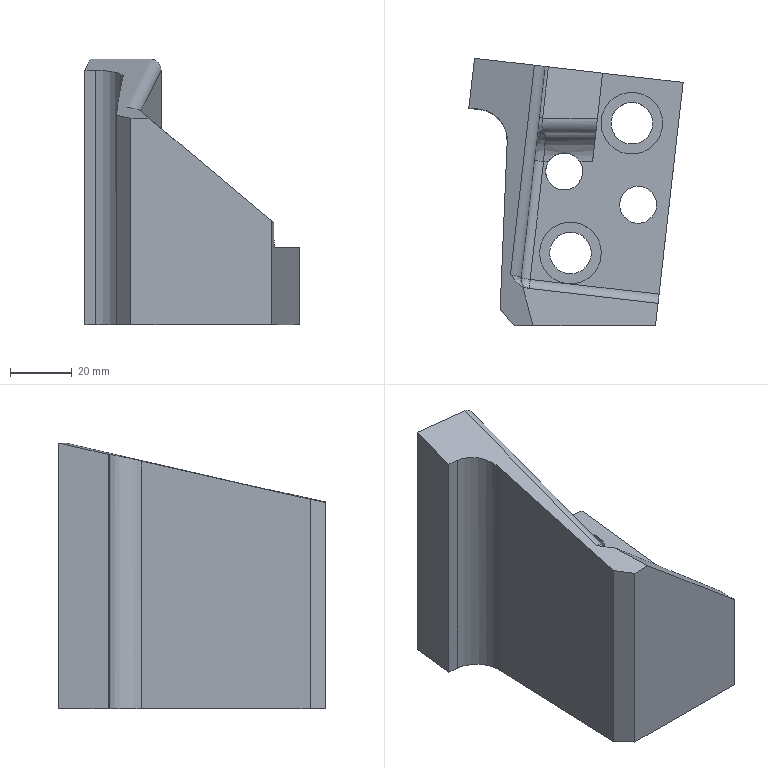Part | NX | features 23 2 | 1 solid | 37 faces | box 69.395 x 86.433 x 86.097 mm | volume 170408 mm3 | plane 18 | cylinder 15 | spline 3 | sphere 1 | commonest cylinder face diameters 6 x5 20 x3 12.001 x2 13.5 x2 7 x1 10 x1
STEP:
#1=CARTESIAN_POINT('',(3804.577,-393.184,-138.));
#2=VERTEX_POINT('',#1);
#3=CARTESIAN_POINT('',(3804.577,-393.184,-104.287));
#4=VERTEX_POINT('',#3);
#5=CARTESIAN_POINT('',(3804.577,-393.184,-83.583));
#6=DIRECTION('',(-0.000000001,0.,1.));
#7=VECTOR('',#6,1000.);
#8=LINE('',#5,#7);
#9=EDGE_CURVE('',#2,#4,#8,.T.);
#10=ORIENTED_EDGE('',*,*,#9,.F.);
#11=CARTESIAN_POINT('',(3813.548,-314.448,-138.));
#12=VERTEX_POINT('',#11);
#13=CARTESIAN_POINT('',(3842.238,-62.642,-138.));
#14=DIRECTION('',(0.1132,0.9936,0.));
#15=VECTOR('',#14,1000.);
#16=LINE('',#13,#15);
#17=EDGE_CURVE('',#2,#12,#16,.T.);
#18=ORIENTED_EDGE('',*,*,#17,.T.);
#19=CARTESIAN_POINT('',(3813.548,-314.448,-113.));
#20=VERTEX_POINT('',#19);
#21=CARTESIAN_POINT('',(3813.548,-314.448,-100.995));
#22=DIRECTION('',(0.000000001,0.,-1.));
#23=VECTOR('',#22,1000.);
#24=LINE('',#21,#23);
#25=EDGE_CURVE('',#20,#12,#24,.T.);
#26=ORIENTED_EDGE('',*,*,#25,.F.);
#27=CARTESIAN_POINT('',(3805.737,-383.004,-113.));
#28=VERTEX_POINT('',#27);
#29=CARTESIAN_POINT('',(3817.039,-283.812,-113.));
#30=DIRECTION('',(0.1132,0.9936,0.));
#31=VECTOR('',#30,1000.);
#32=LINE('',#29,#31);
#33=EDGE_CURVE('',#28,#20,#32,.T.);
#34=ORIENTED_EDGE('',*,*,#33,.F.);
#35=CARTESIAN_POINT('',(3805.397,-385.985,-110.));
#36=VERTEX_POINT('',#35);
#37=CARTESIAN_POINT('',(3805.737,-383.004,-110.));
#38=DIRECTION('',(-0.9936,0.1132,-0.000000001));
#39=DIRECTION('',(-0.1132,-0.9936,0.));
#40=AXIS2_PLACEMENT_3D('',#37,#38,#39);
#41=CIRCLE('',#40,3.);
#42=EDGE_CURVE('',#28,#36,#41,.T.);
#43=ORIENTED_EDGE('',*,*,#42,.T.);
#44=CARTESIAN_POINT('',(3805.397,-385.985,-104.975));
#45=VERTEX_POINT('',#44);
#46=CARTESIAN_POINT('',(3805.397,-385.985,-102.134));
#47=DIRECTION('',(0.000000001,0.,-1.));
#48=VECTOR('',#47,1000.);
#49=LINE('',#46,#48);
#50=EDGE_CURVE('',#45,#36,#49,.T.);
#51=ORIENTED_EDGE('',*,*,#50,.F.);
#52=CARTESIAN_POINT('',(3792.366,-500.365,-94.04));
#53=DIRECTION('',(-0.1127,-0.9891,0.09456));
#54=VECTOR('',#53,1000.);
#55=LINE('',#52,#54);
#56=EDGE_CURVE('',#45,#4,#55,.T.);
#57=ORIENTED_EDGE('',*,*,#56,.T.);
#58=EDGE_LOOP('',(#10,#18,#26,#34,#43,#51,#57));
#59=FACE_BOUND('',#58,.T.);
#60=CARTESIAN_POINT('',(3817.039,-283.812,-83.583));
#61=DIRECTION('',(-0.9936,0.1132,-0.000000001));
#62=DIRECTION('',(0.1132,0.9936,0.));
#63=AXIS2_PLACEMENT_3D('',#60,#61,#62);
#64=PLANE('',#63);
#65=ADVANCED_FACE('',(#59),#64,.F.);
#66=CARTESIAN_POINT('',(3754.275,-388.188,-138.));
#67=VERTEX_POINT('',#66);
#68=CARTESIAN_POINT('',(3756.561,-333.591,-138.));
#69=VERTEX_POINT('',#68);
#70=CARTESIAN_POINT('',(3774.796,101.868,-138.));
#71=DIRECTION('',(0.04184,0.9991,0.));
#72=VECTOR('',#71,1000.);
#73=LINE('',#70,#72);
#74=EDGE_CURVE('',#67,#69,#73,.T.);
#75=ORIENTED_EDGE('',*,*,#74,.F.);
#76=CARTESIAN_POINT('',(3754.275,-388.188,-70.123));
#77=VERTEX_POINT('',#76);
#78=CARTESIAN_POINT('',(3754.275,-388.188,-382.321));
#79=DIRECTION('',(0.,0.,1.));
#80=VECTOR('',#79,1000.);
#81=LINE('',#78,#80);
#82=EDGE_CURVE('',#67,#77,#81,.T.);
#83=ORIENTED_EDGE('',*,*,#82,.T.);
#84=CARTESIAN_POINT('',(3756.561,-333.591,-57.705));
#85=VERTEX_POINT('',#84);
#86=CARTESIAN_POINT('',(3754.968,-371.632,-66.358));
#87=DIRECTION('',(0.0408,0.9743,0.2216));
#88=VECTOR('',#87,1000.);
#89=LINE('',#86,#88);
#90=EDGE_CURVE('',#77,#85,#89,.T.);
#91=ORIENTED_EDGE('',*,*,#90,.T.);
#92=CARTESIAN_POINT('',(3756.561,-333.591,-133.));
#93=DIRECTION('',(0.,0.,-1.));
#94=VECTOR('',#93,1000.);
#95=LINE('',#92,#94);
#96=EDGE_CURVE('',#85,#69,#95,.T.);
#97=ORIENTED_EDGE('',*,*,#96,.T.);
#98=EDGE_LOOP('',(#75,#83,#91,#97));
#99=FACE_BOUND('',#98,.T.);
#100=CARTESIAN_POINT('',(3759.776,-256.811,-382.321));
#101=DIRECTION('',(-0.9991,0.04184,0.));
#102=DIRECTION('',(0.04184,0.9991,0.));
#103=AXIS2_PLACEMENT_3D('',#100,#101,#102);
#104=PLANE('',#103);
#105=ADVANCED_FACE('',(#99),#104,.T.);
#106=ORIENTED_EDGE('',*,*,#90,.F.);
#107=CARTESIAN_POINT('',(3759.066,-393.184,-71.13));
#108=VERTEX_POINT('',#107);
#109=CARTESIAN_POINT('',(3785.069,-420.298,-76.597));
#110=DIRECTION('',(0.6849,-0.7142,-0.144));
#111=VECTOR('',#110,1000.);
#112=LINE('',#109,#111);
#113=EDGE_CURVE('',#77,#108,#112,.T.);
#114=ORIENTED_EDGE('',*,*,#113,.T.);
#115=CARTESIAN_POINT('',(3764.884,-393.184,-70.98));
#116=VERTEX_POINT('',#115);
#117=CARTESIAN_POINT('',(3765.334,-393.184,-70.968));
#118=DIRECTION('',(-0.9997,0.,-0.02578));
#119=VECTOR('',#118,1000.);
#120=LINE('',#117,#119);
#121=EDGE_CURVE('',#116,#108,#120,.T.);
#122=ORIENTED_EDGE('',*,*,#121,.F.);
#123=CARTESIAN_POINT('',(3761.625,-380.732,-68.246));
#124=VERTEX_POINT('',#123);
#125=CARTESIAN_POINT('',(3784.867,-469.535,-87.747));
#126=DIRECTION('',(-0.2477,0.9463,0.2078));
#127=VECTOR('',#126,1000.);
#128=LINE('',#125,#127);
#129=EDGE_CURVE('',#116,#124,#128,.T.);
#130=ORIENTED_EDGE('',*,*,#129,.T.);
#131=CARTESIAN_POINT('',(3757.624,-376.852,-67.47));
#132=VERTEX_POINT('',#131);
#133=CARTESIAN_POINT('',(3761.625,-380.732,-68.246));
#134=CARTESIAN_POINT('',(3761.272,-380.557,-68.215));
#135=CARTESIAN_POINT('',(3760.738,-380.211,-68.151));
#136=CARTESIAN_POINT('',(3760.089,-379.642,-68.038));
#137=CARTESIAN_POINT('',(3759.731,-379.291,-67.968));
#138=CARTESIAN_POINT('',(3759.413,-378.954,-67.9));
#139=CARTESIAN_POINT('',(3759.272,-378.795,-67.868));
#140=CARTESIAN_POINT('',(3758.967,-378.446,-67.797));
#141=CARTESIAN_POINT('',(3758.665,-378.087,-67.723));
#142=CARTESIAN_POINT('',(3758.18,-377.503,-67.603));
#143=CARTESIAN_POINT('',(3757.844,-377.103,-67.522));
#144=CARTESIAN_POINT('',(3757.683,-376.916,-67.483));
#145=CARTESIAN_POINT('',(3757.624,-376.852,-67.47));
#146=B_SPLINE_CURVE_WITH_KNOTS('',3,(#133,#134,#135,#136,#137,#138,#139,#140,#141,#142,#143,#144,#145),.UNSPECIFIED.,.F.,.F.,(4,1,1,1,1,1,1,1,1,1,4),(0.,0.25,0.375,0.4375,0.5,0.5625,0.625,0.75,0.8125,0.875,1.),.UNSPECIFIED.);
#147=EDGE_CURVE('',#124,#132,#146,.T.);
#148=ORIENTED_EDGE('',*,*,#147,.T.);
#149=CARTESIAN_POINT('',(3765.36,-308.958,-51.903));
#150=VERTEX_POINT('',#149);
#151=CARTESIAN_POINT('',(3758.256,-371.305,-66.199));
#152=DIRECTION('',(-0.1104,-0.9687,-0.2221));
#153=VECTOR('',#152,1000.);
#154=LINE('',#151,#153);
#155=EDGE_CURVE('',#150,#132,#154,.T.);
#156=ORIENTED_EDGE('',*,*,#155,.F.);
#157=CARTESIAN_POINT('',(3745.985,-306.75,-51.903));
#158=VERTEX_POINT('',#157);
#159=CARTESIAN_POINT('',(3772.315,-309.75,-51.903));
#160=DIRECTION('',(0.9936,-0.1132,-0.000000001));
#161=VECTOR('',#160,1000.);
#162=LINE('',#159,#161);
#163=EDGE_CURVE('',#158,#150,#162,.T.);
#164=ORIENTED_EDGE('',*,*,#163,.F.);
#165=CARTESIAN_POINT('',(3744.153,-322.832,-55.59));
#166=VERTEX_POINT('',#165);
#167=CARTESIAN_POINT('',(3738.882,-369.098,-66.199));
#168=DIRECTION('',(-0.1104,-0.9687,-0.2221));
#169=VECTOR('',#168,1000.);
#170=LINE('',#167,#169);
#171=EDGE_CURVE('',#158,#166,#170,.T.);
#172=ORIENTED_EDGE('',*,*,#171,.T.);
#173=CARTESIAN_POINT('',(3747.702,-323.236,-55.59));
#174=VERTEX_POINT('',#173);
#175=CARTESIAN_POINT('',(3737.198,-322.04,-55.59));
#176=DIRECTION('',(0.9936,-0.1132,-0.000000001));
#177=VECTOR('',#176,1000.);
#178=LINE('',#175,#177);
#179=EDGE_CURVE('',#166,#174,#178,.T.);
#180=ORIENTED_EDGE('',*,*,#179,.T.);
#181=CARTESIAN_POINT('',(3746.57,-333.172,-57.868));
#182=DIRECTION('',(0.02515,0.2207,-0.975));
#183=DIRECTION('',(0.1104,0.9687,0.2221));
#184=AXIS2_PLACEMENT_3D('',#181,#182,#183);
#185=ELLIPSE('',#184,10.256,10.);
#186=EDGE_CURVE('',#174,#85,#185,.T.);
#187=ORIENTED_EDGE('',*,*,#186,.T.);
#188=EDGE_LOOP('',(#106,#114,#122,#130,#148,#156,#164,#172,#180,#187));
#189=FACE_BOUND('',#188,.T.);
#190=CARTESIAN_POINT('',(3765.211,-372.098,-66.199));
#191=DIRECTION('',(0.02515,0.2207,-0.975));
#192=DIRECTION('',(-0.1104,-0.9687,-0.2221));
#193=AXIS2_PLACEMENT_3D('',#190,#191,#192);
#194=PLANE('',#193);
#195=ADVANCED_FACE('',(#189),#194,.F.);
#196=CARTESIAN_POINT('',(3790.196,-327.653,-138.));
#197=VERTEX_POINT('',#196);
#198=CARTESIAN_POINT('',(3796.946,-327.653,-138.));
#199=DIRECTION('',(0.,0.,-1.));
#200=DIRECTION('',(-1.,0.,0.));
#201=AXIS2_PLACEMENT_3D('',#198,#199,#200);
#202=CIRCLE('',#201,6.75);
#203=EDGE_CURVE('',#197,#197,#202,.T.);
#204=ORIENTED_EDGE('',*,*,#203,.F.);
#205=EDGE_LOOP('',(#204));
#206=FACE_BOUND('',#205,.T.);
#207=CARTESIAN_POINT('',(3769.037,-343.274,-138.));
#208=VERTEX_POINT('',#207);
#209=CARTESIAN_POINT('',(3775.037,-343.274,-138.));
#210=DIRECTION('',(0.,0.,-1.));
#211=DIRECTION('',(-1.,0.,0.));
#212=AXIS2_PLACEMENT_3D('',#209,#210,#211);
#213=CIRCLE('',#212,6.);
#214=EDGE_CURVE('',#208,#208,#213,.T.);
#215=ORIENTED_EDGE('',*,*,#214,.F.);
#216=EDGE_LOOP('',(#215));
#217=FACE_BOUND('',#216,.T.);
#218=CARTESIAN_POINT('',(3792.971,-354.052,-138.));
#219=VERTEX_POINT('',#218);
#220=CARTESIAN_POINT('',(3798.971,-354.052,-138.));
#221=DIRECTION('',(0.,0.,-1.));
#222=DIRECTION('',(-1.,0.,0.));
#223=AXIS2_PLACEMENT_3D('',#220,#221,#222);
#224=CIRCLE('',#223,6.);
#225=EDGE_CURVE('',#219,#219,#224,.T.);
#226=ORIENTED_EDGE('',*,*,#225,.F.);
#227=EDGE_LOOP('',(#226));
#228=FACE_BOUND('',#227,.T.);
#229=CARTESIAN_POINT('',(3770.312,-369.673,-138.));
#230=VERTEX_POINT('',#229);
#231=CARTESIAN_POINT('',(3777.062,-369.673,-138.));
#232=DIRECTION('',(0.,0.,-1.));
#233=DIRECTION('',(-1.,0.,0.));
#234=AXIS2_PLACEMENT_3D('',#231,#232,#233);
#235=CIRCLE('',#234,6.75);
#236=EDGE_CURVE('',#230,#230,#235,.T.);
#237=ORIENTED_EDGE('',*,*,#236,.F.);
#238=EDGE_LOOP('',(#237));
#239=FACE_BOUND('',#238,.T.);
#240=CARTESIAN_POINT('',(3759.066,-393.184,-138.));
#241=VERTEX_POINT('',#240);
#242=CARTESIAN_POINT('',(1598.5,-393.184,-138.));
#243=DIRECTION('',(-1.,0.,0.));
#244=VECTOR('',#243,1000.);
#245=LINE('',#242,#244);
#246=EDGE_CURVE('',#2,#241,#245,.T.);
#247=ORIENTED_EDGE('',*,*,#246,.T.);
#248=CARTESIAN_POINT('',(2431.145,991.508,-138.));
#249=DIRECTION('',(-0.6922,0.7217,0.));
#250=VECTOR('',#249,1000.);
#251=LINE('',#248,#250);
#252=EDGE_CURVE('',#241,#67,#251,.T.);
#253=ORIENTED_EDGE('',*,*,#252,.T.);
#254=ORIENTED_EDGE('',*,*,#74,.T.);
#255=CARTESIAN_POINT('',(3747.702,-323.236,-138.));
#256=VERTEX_POINT('',#255);
#257=CARTESIAN_POINT('',(3746.57,-333.172,-138.));
#258=DIRECTION('',(0.,0.,1.));
#259=DIRECTION('',(-1.,0.,0.));
#260=AXIS2_PLACEMENT_3D('',#257,#258,#259);
#261=CIRCLE('',#260,10.);
#262=EDGE_CURVE('',#69,#256,#261,.T.);
#263=ORIENTED_EDGE('',*,*,#262,.T.);
#264=CARTESIAN_POINT('',(3744.153,-322.832,-138.));
#265=VERTEX_POINT('',#264);
#266=CARTESIAN_POINT('',(3737.198,-322.04,-138.));
#267=DIRECTION('',(0.9936,-0.1132,0.));
#268=VECTOR('',#267,1000.);
#269=LINE('',#266,#268);
#270=EDGE_CURVE('',#265,#256,#269,.T.);
#271=ORIENTED_EDGE('',*,*,#270,.F.);
#272=CARTESIAN_POINT('',(3745.985,-306.75,-138.));
#273=VERTEX_POINT('',#272);
#274=CARTESIAN_POINT('',(3774.675,-54.944,-138.));
#275=DIRECTION('',(-0.1132,-0.9936,0.));
#276=VECTOR('',#275,1000.);
#277=LINE('',#274,#276);
#278=EDGE_CURVE('',#273,#265,#277,.T.);
#279=ORIENTED_EDGE('',*,*,#278,.F.);
#280=CARTESIAN_POINT('',(1569.81,-58.806,-138.));
#281=DIRECTION('',(0.9936,-0.1132,0.));
#282=VECTOR('',#281,1000.);
#283=LINE('',#280,#282);
#284=EDGE_CURVE('',#273,#12,#283,.T.);
#285=ORIENTED_EDGE('',*,*,#284,.T.);
#286=ORIENTED_EDGE('',*,*,#17,.F.);
#287=EDGE_LOOP('',(#247,#253,#254,#263,#271,#279,#285,#286));
#288=FACE_BOUND('',#287,.T.);
#289=CARTESIAN_POINT('',(1598.5,193.,-138.));
#290=DIRECTION('',(0.,0.,-1.));
#291=DIRECTION('',(-1.,0.,0.));
#292=AXIS2_PLACEMENT_3D('',#289,#290,#291);
#293=PLANE('',#292);
#294=ADVANCED_FACE('',(#206,#217,#228,#239,#288),#293,.T.);
#295=ORIENTED_EDGE('',*,*,#129,.F.);
#296=CARTESIAN_POINT('',(3738.981,-393.184,-49.245));
#297=DIRECTION('',(0.766,0.,-0.6428));
#298=VECTOR('',#297,1000.);
#299=LINE('',#296,#298);
#300=EDGE_CURVE('',#116,#4,#299,.T.);
#301=ORIENTED_EDGE('',*,*,#300,.T.);
#302=ORIENTED_EDGE('',*,*,#56,.F.);
#303=CARTESIAN_POINT('',(3763.53,-381.215,-69.844));
#304=VERTEX_POINT('',#303);
#305=CARTESIAN_POINT('',(3746.385,-379.261,-55.457));
#306=DIRECTION('',(0.7631,-0.08695,-0.6404));
#307=VECTOR('',#306,1000.);
#308=LINE('',#305,#307);
#309=EDGE_CURVE('',#304,#45,#308,.T.);
#310=ORIENTED_EDGE('',*,*,#309,.F.);
#311=CARTESIAN_POINT('',(3763.53,-381.215,-69.844));
#312=CARTESIAN_POINT('',(3762.882,-381.141,-69.3));
#313=CARTESIAN_POINT('',(3762.255,-380.926,-68.774));
#314=CARTESIAN_POINT('',(3761.625,-380.733,-68.245));
#315=B_SPLINE_CURVE_WITH_KNOTS('',3,(#311,#312,#313,#314),.UNSPECIFIED.,.F.,.F.,(4,4),(0.,0.002533),.UNSPECIFIED.);
#316=EDGE_CURVE('',#304,#124,#315,.T.);
#317=ORIENTED_EDGE('',*,*,#316,.T.);
#318=EDGE_LOOP('',(#295,#301,#302,#310,#317));
#319=FACE_BOUND('',#318,.T.);
#320=CARTESIAN_POINT('',(3738.981,-490.,-49.245));
#321=DIRECTION('',(0.6428,0.,0.766));
#322=DIRECTION('',(-0.766,0.,0.6428));
#323=AXIS2_PLACEMENT_3D('',#320,#321,#322);
#324=PLANE('',#323);
#325=ADVANCED_FACE('',(#319),#324,.T.);
#326=CARTESIAN_POINT('',(3786.946,-327.653,-128.));
#327=VERTEX_POINT('',#326);
#328=CARTESIAN_POINT('',(3796.946,-327.653,-128.));
#329=DIRECTION('',(0.,0.,-1.));
#330=DIRECTION('',(-1.,0.,0.));
#331=AXIS2_PLACEMENT_3D('',#328,#329,#330);
#332=CIRCLE('',#331,10.);
#333=EDGE_CURVE('',#327,#327,#332,.T.);
#334=ORIENTED_EDGE('',*,*,#333,.T.);
#335=EDGE_LOOP('',(#334));
#336=FACE_BOUND('',#335,.T.);
#337=CARTESIAN_POINT('',(3786.946,-327.653,-113.));
#338=VERTEX_POINT('',#337);
#339=CARTESIAN_POINT('',(3796.946,-327.653,-113.));
#340=DIRECTION('',(0.,0.,1.));
#341=DIRECTION('',(-1.,0.,0.));
#342=AXIS2_PLACEMENT_3D('',#339,#340,#341);
#343=CIRCLE('',#342,10.);
#344=EDGE_CURVE('',#338,#338,#343,.T.);
#345=ORIENTED_EDGE('',*,*,#344,.T.);
#346=EDGE_LOOP('',(#345));
#347=FACE_BOUND('',#346,.T.);
#348=CARTESIAN_POINT('',(3796.946,-327.653,-103.074));
#349=DIRECTION('',(0.,0.,-1.));
#350=DIRECTION('',(-1.,0.,0.));
#351=AXIS2_PLACEMENT_3D('',#348,#349,#350);
#352=CYLINDRICAL_SURFACE('',#351,10.);
#353=ADVANCED_FACE('',(#336,#347),#352,.F.);
#354=ORIENTED_EDGE('',*,*,#344,.F.);
#355=EDGE_LOOP('',(#354));
#356=FACE_BOUND('',#355,.T.);
#357=CARTESIAN_POINT('',(3792.971,-354.052,-113.));
#358=VERTEX_POINT('',#357);
#359=CARTESIAN_POINT('',(3798.971,-354.052,-113.));
#360=DIRECTION('',(0.,0.,1.));
#361=DIRECTION('',(-1.,0.,0.));
#362=AXIS2_PLACEMENT_3D('',#359,#360,#361);
#363=CIRCLE('',#362,6.);
#364=EDGE_CURVE('',#358,#358,#363,.T.);
#365=ORIENTED_EDGE('',*,*,#364,.F.);
#366=EDGE_LOOP('',(#365));
#367=FACE_BOUND('',#366,.T.);
#368=CARTESIAN_POINT('',(3768.354,-340.096,-113.));
#369=VERTEX_POINT('',#368);
#370=CARTESIAN_POINT('',(3769.947,-340.096,-113.));
#371=VERTEX_POINT('',#370);
#372=CARTESIAN_POINT('',(282.5,-340.096,-113.));
#373=DIRECTION('',(1.,0.,0.));
#374=VECTOR('',#373,1000.);
#375=LINE('',#372,#374);
#376=EDGE_CURVE('',#369,#371,#375,.T.);
#377=ORIENTED_EDGE('',*,*,#376,.F.);
#378=CARTESIAN_POINT('',(3764.007,-378.25,-113.));
#379=VERTEX_POINT('',#378);
#380=CARTESIAN_POINT('',(3764.007,-378.25,-113.));
#381=DIRECTION('',(-0.1132,-0.9936,0.));
#382=VECTOR('',#381,1000.);
#383=LINE('',#380,#382);
#384=EDGE_CURVE('',#369,#379,#383,.T.);
#385=ORIENTED_EDGE('',*,*,#384,.T.);
#386=CARTESIAN_POINT('',(3775.93,-379.608,-113.));
#387=VERTEX_POINT('',#386);
#388=CARTESIAN_POINT('',(262.864,20.655,-113.));
#389=DIRECTION('',(0.9936,-0.1132,0.));
#390=VECTOR('',#389,1000.);
#391=LINE('',#388,#390);
#392=EDGE_CURVE('',#379,#387,#391,.T.);
#393=ORIENTED_EDGE('',*,*,#392,.T.);
#394=CARTESIAN_POINT('',(3777.062,-369.673,-113.));
#395=DIRECTION('',(0.,0.,1.));
#396=DIRECTION('',(-1.,0.,0.));
#397=AXIS2_PLACEMENT_3D('',#394,#395,#396);
#398=CIRCLE('',#397,10.);
#399=EDGE_CURVE('',#387,#387,#398,.T.);
#400=ORIENTED_EDGE('',*,*,#399,.F.);
#401=CARTESIAN_POINT('',(262.864,20.655,-113.));
#402=DIRECTION('',(0.9936,-0.1132,0.));
#403=VECTOR('',#402,1000.);
#404=LINE('',#401,#403);
#405=EDGE_CURVE('',#387,#28,#404,.T.);
#406=ORIENTED_EDGE('',*,*,#405,.T.);
#407=ORIENTED_EDGE('',*,*,#33,.T.);
#408=CARTESIAN_POINT('',(3787.453,-311.475,-113.));
#409=VERTEX_POINT('',#408);
#410=CARTESIAN_POINT('',(3780.809,-310.718,-113.));
#411=DIRECTION('',(-0.9936,0.1132,0.));
#412=VECTOR('',#411,1000.);
#413=LINE('',#410,#412);
#414=EDGE_CURVE('',#20,#409,#413,.T.);
#415=ORIENTED_EDGE('',*,*,#414,.T.);
#416=CARTESIAN_POINT('',(3784.192,-340.096,-113.));
#417=VERTEX_POINT('',#416);
#418=CARTESIAN_POINT('',(3799.278,-207.685,-113.));
#419=DIRECTION('',(-0.1132,-0.9936,0.));
#420=VECTOR('',#419,1000.);
#421=LINE('',#418,#420);
#422=EDGE_CURVE('',#409,#417,#421,.T.);
#423=ORIENTED_EDGE('',*,*,#422,.T.);
#424=CARTESIAN_POINT('',(3780.128,-340.096,-113.));
#425=VERTEX_POINT('',#424);
#426=CARTESIAN_POINT('',(282.5,-340.096,-113.));
#427=DIRECTION('',(1.,0.,0.));
#428=VECTOR('',#427,1000.);
#429=LINE('',#426,#428);
#430=EDGE_CURVE('',#425,#417,#429,.T.);
#431=ORIENTED_EDGE('',*,*,#430,.F.);
#432=CARTESIAN_POINT('',(3775.037,-343.274,-113.));
#433=DIRECTION('',(0.,0.,1.));
#434=DIRECTION('',(-1.,0.,0.));
#435=AXIS2_PLACEMENT_3D('',#432,#433,#434);
#436=CIRCLE('',#435,6.);
#437=EDGE_CURVE('',#371,#425,#436,.T.);
#438=ORIENTED_EDGE('',*,*,#437,.F.);
#439=EDGE_LOOP('',(#377,#385,#393,#400,#406,#407,#415,#423,#431,#438));
#440=FACE_BOUND('',#439,.T.);
#441=CARTESIAN_POINT('',(282.5,193.,-113.));
#442=DIRECTION('',(0.,0.,-1.));
#443=DIRECTION('',(-1.,0.,0.));
#444=AXIS2_PLACEMENT_3D('',#441,#442,#443);
#445=PLANE('',#444);
#446=ADVANCED_FACE('',(#356,#367,#440),#445,.F.);
#447=CARTESIAN_POINT('',(3787.453,-311.475,-91.917));
#448=VERTEX_POINT('',#447);
#449=CARTESIAN_POINT('',(3769.914,-309.477,-77.201));
#450=VERTEX_POINT('',#449);
#451=CARTESIAN_POINT('',(3788.947,-311.645,-93.171));
#452=DIRECTION('',(-0.7631,0.08695,0.6404));
#453=VECTOR('',#452,1000.);
#454=LINE('',#451,#453);
#455=EDGE_CURVE('',#448,#450,#454,.T.);
#456=ORIENTED_EDGE('',*,*,#455,.T.);
#457=CARTESIAN_POINT('',(3768.021,-326.096,-75.612));
#458=VERTEX_POINT('',#457);
#459=CARTESIAN_POINT('',(3635.355,-1490.486,35.707));
#460=DIRECTION('',(-0.1127,-0.9891,0.09456));
#461=VECTOR('',#460,1000.);
#462=LINE('',#459,#461);
#463=EDGE_CURVE('',#450,#458,#462,.T.);
#464=ORIENTED_EDGE('',*,*,#463,.T.);
#465=CARTESIAN_POINT('',(3785.787,-326.096,-90.52));
#466=VERTEX_POINT('',#465);
#467=CARTESIAN_POINT('',(3738.981,-326.096,-51.245));
#468=DIRECTION('',(0.766,0.,-0.6428));
#469=VECTOR('',#468,1000.);
#470=LINE('',#467,#469);
#471=EDGE_CURVE('',#458,#466,#470,.T.);
#472=ORIENTED_EDGE('',*,*,#471,.T.);
#473=CARTESIAN_POINT('',(3766.504,-495.344,-74.339));
#474=DIRECTION('',(-0.1127,-0.9891,0.09456));
#475=VECTOR('',#474,1000.);
#476=LINE('',#473,#475);
#477=EDGE_CURVE('',#448,#466,#476,.T.);
#478=ORIENTED_EDGE('',*,*,#477,.F.);
#479=EDGE_LOOP('',(#456,#464,#472,#478));
#480=FACE_BOUND('',#479,.T.);
#481=CARTESIAN_POINT('',(3738.981,-490.,-51.245));
#482=DIRECTION('',(0.6428,0.,0.766));
#483=DIRECTION('',(-0.766,0.,0.6428));
#484=AXIS2_PLACEMENT_3D('',#481,#482,#483);
#485=PLANE('',#484);
#486=ADVANCED_FACE('',(#480),#485,.T.);
#487=CARTESIAN_POINT('',(3787.453,-311.475,-100.995));
#488=DIRECTION('',(0.,0.,-1.));
#489=VECTOR('',#488,1000.);
#490=LINE('',#487,#489);
#491=EDGE_CURVE('',#448,#409,#490,.T.);
#492=ORIENTED_EDGE('',*,*,#491,.T.);
#493=ORIENTED_EDGE('',*,*,#414,.F.);
#494=ORIENTED_EDGE('',*,*,#25,.T.);
#495=ORIENTED_EDGE('',*,*,#284,.F.);
#496=CARTESIAN_POINT('',(3745.985,-306.75,-706.6));
#497=DIRECTION('',(0.000000001,0.,-1.));
#498=VECTOR('',#497,1000.);
#499=LINE('',#496,#498);
#500=EDGE_CURVE('',#158,#273,#499,.T.);
#501=ORIENTED_EDGE('',*,*,#500,.F.);
#502=ORIENTED_EDGE('',*,*,#163,.T.);
#503=CARTESIAN_POINT('',(3768.837,-309.354,-55.492));
#504=VERTEX_POINT('',#503);
#505=CARTESIAN_POINT('',(3765.36,-308.958,-55.492));
#506=DIRECTION('',(-0.1132,-0.9936,0.));
#507=DIRECTION('',(0.,0.,1.));
#508=AXIS2_PLACEMENT_3D('',#505,#506,#507);
#509=ELLIPSE('',#508,3.59,3.5);
#510=EDGE_CURVE('',#504,#150,#509,.T.);
#511=ORIENTED_EDGE('',*,*,#510,.F.);
#512=CARTESIAN_POINT('',(3768.837,-309.354,-74.882));
#513=VERTEX_POINT('',#512);
#514=CARTESIAN_POINT('',(3768.837,-309.354,-706.6));
#515=DIRECTION('',(-0.000000001,0.,1.));
#516=VECTOR('',#515,1000.);
#517=LINE('',#514,#516);
#518=EDGE_CURVE('',#513,#504,#517,.T.);
#519=ORIENTED_EDGE('',*,*,#518,.F.);
#520=CARTESIAN_POINT('',(3771.818,-309.693,-74.882));
#521=DIRECTION('',(-0.1132,-0.9936,0.));
#522=DIRECTION('',(-0.000000001,0.,1.));
#523=AXIS2_PLACEMENT_3D('',#520,#521,#522);
#524=ELLIPSE('',#523,3.014,3.);
#525=EDGE_CURVE('',#513,#450,#524,.T.);
#526=ORIENTED_EDGE('',*,*,#525,.T.);
#527=ORIENTED_EDGE('',*,*,#455,.F.);
#528=EDGE_LOOP('',(#492,#493,#494,#495,#501,#502,#511,#519,#526,#527));
#529=FACE_BOUND('',#528,.T.);
#530=CARTESIAN_POINT('',(3780.809,-310.718,-100.995));
#531=DIRECTION('',(-0.1132,-0.9936,0.));
#532=DIRECTION('',(-0.9936,0.1132,0.));
#533=AXIS2_PLACEMENT_3D('',#530,#531,#532);
#534=PLANE('',#533);
#535=ADVANCED_FACE('',(#529),#534,.F.);
#536=CARTESIAN_POINT('',(3785.217,-331.096,-96.569));
#537=VERTEX_POINT('',#536);
#538=CARTESIAN_POINT('',(3769.038,-331.096,-82.992));
#539=VERTEX_POINT('',#538);
#540=CARTESIAN_POINT('',(3769.312,-331.096,-83.222));
#541=DIRECTION('',(-0.766,0.,0.6428));
#542=VECTOR('',#541,1000.);
#543=LINE('',#540,#542);
#544=EDGE_CURVE('',#537,#539,#543,.T.);
#545=ORIENTED_EDGE('',*,*,#544,.T.);
#546=CARTESIAN_POINT('',(3769.038,-331.096,-104.));
#547=VERTEX_POINT('',#546);
#548=CARTESIAN_POINT('',(3769.038,-331.096,-104.));
#549=DIRECTION('',(0.000000001,0.,-1.));
#550=VECTOR('',#549,1000.);
#551=LINE('',#548,#550);
#552=EDGE_CURVE('',#539,#547,#551,.T.);
#553=ORIENTED_EDGE('',*,*,#552,.T.);
#554=CARTESIAN_POINT('',(3785.217,-331.096,-104.));
#555=VERTEX_POINT('',#554);
#556=CARTESIAN_POINT('',(3769.38,-331.096,-104.));
#557=DIRECTION('',(1.,0.,0.));
#558=VECTOR('',#557,1000.);
#559=LINE('',#556,#558);
#560=EDGE_CURVE('',#547,#555,#559,.T.);
#561=ORIENTED_EDGE('',*,*,#560,.T.);
#562=CARTESIAN_POINT('',(3785.217,-331.096,-81.141));
#563=DIRECTION('',(0.,0.,-1.));
#564=VECTOR('',#563,1000.);
#565=LINE('',#562,#564);
#566=EDGE_CURVE('',#537,#555,#565,.T.);
#567=ORIENTED_EDGE('',*,*,#566,.F.);
#568=EDGE_LOOP('',(#545,#553,#561,#567));
#569=FACE_BOUND('',#568,.T.);
#570=CARTESIAN_POINT('',(3769.38,-331.096,-81.141));
#571=DIRECTION('',(0.,-1.,0.));
#572=DIRECTION('',(0.,0.,1.));
#573=AXIS2_PLACEMENT_3D('',#570,#571,#572);
#574=PLANE('',#573);
#575=ADVANCED_FACE('',(#569),#574,.T.);
#576=CARTESIAN_POINT('',(3761.026,-377.91,-71.212));
#577=VERTEX_POINT('',#576);
#578=CARTESIAN_POINT('',(3617.366,-1638.801,-360.329));
#579=DIRECTION('',(0.1104,0.9687,0.2221));
#580=VECTOR('',#579,1000.);
#581=LINE('',#578,#580);
#582=EDGE_CURVE('',#577,#504,#581,.T.);
#583=ORIENTED_EDGE('',*,*,#582,.F.);
#584=CARTESIAN_POINT('',(3761.026,-377.91,-110.));
#585=VERTEX_POINT('',#584);
#586=CARTESIAN_POINT('',(3761.026,-377.91,-706.6));
#587=DIRECTION('',(0.000000001,0.,-1.));
#588=VECTOR('',#587,1000.);
#589=LINE('',#586,#588);
#590=EDGE_CURVE('',#577,#585,#589,.T.);
#591=ORIENTED_EDGE('',*,*,#590,.T.);
#592=CARTESIAN_POINT('',(3765.373,-339.757,-110.));
#593=VERTEX_POINT('',#592);
#594=CARTESIAN_POINT('',(3626.296,-1560.421,-110.));
#595=DIRECTION('',(0.1132,0.9936,0.));
#596=VECTOR('',#595,1000.);
#597=LINE('',#594,#596);
#598=EDGE_CURVE('',#585,#593,#597,.T.);
#599=ORIENTED_EDGE('',*,*,#598,.T.);
#600=CARTESIAN_POINT('',(3766.057,-333.757,-104.));
#601=VERTEX_POINT('',#600);
#602=CARTESIAN_POINT('',(3765.373,-339.757,-104.));
#603=DIRECTION('',(0.9936,-0.1132,0.000000001));
#604=DIRECTION('',(0.1132,0.9936,-0.000000007));
#605=AXIS2_PLACEMENT_3D('',#602,#603,#604);
#606=ELLIPSE('',#605,6.039,6.);
#607=EDGE_CURVE('',#593,#601,#606,.T.);
#608=ORIENTED_EDGE('',*,*,#607,.T.);
#609=CARTESIAN_POINT('',(3766.057,-333.757,-82.992));
#610=VERTEX_POINT('',#609);
#611=CARTESIAN_POINT('',(3766.057,-333.757,-78.746));
#612=DIRECTION('',(-0.000000001,0.,1.));
#613=VECTOR('',#612,1000.);
#614=LINE('',#611,#613);
#615=EDGE_CURVE('',#601,#610,#614,.T.);
#616=ORIENTED_EDGE('',*,*,#615,.T.);
#617=CARTESIAN_POINT('',(3766.968,-325.757,-73.314));
#618=VERTEX_POINT('',#617);
#619=CARTESIAN_POINT('',(3766.968,-325.757,-83.757));
#620=DIRECTION('',(-0.9936,0.1132,-0.000000001));
#621=DIRECTION('',(-0.01514,-0.1328,0.991));
#622=AXIS2_PLACEMENT_3D('',#619,#620,#621);
#623=ELLIPSE('',#622,10.511,8.);
#624=EDGE_CURVE('',#610,#618,#623,.T.);
#625=ORIENTED_EDGE('',*,*,#624,.T.);
#626=CARTESIAN_POINT('',(3634.303,-1490.146,38.006));
#627=DIRECTION('',(0.1127,0.9891,-0.09456));
#628=VECTOR('',#627,1000.);
#629=LINE('',#626,#628);
#630=EDGE_CURVE('',#618,#513,#629,.T.);
#631=ORIENTED_EDGE('',*,*,#630,.T.);
#632=ORIENTED_EDGE('',*,*,#518,.T.);
#633=EDGE_LOOP('',(#583,#591,#599,#608,#616,#625,#631,#632));
#634=FACE_BOUND('',#633,.T.);
#635=CARTESIAN_POINT('',(3626.296,-1560.421,-706.6));
#636=DIRECTION('',(0.9936,-0.1132,0.000000001));
#637=DIRECTION('',(0.000000001,0.000000001,-1.));
#638=AXIS2_PLACEMENT_3D('',#635,#636,#637);
#639=PLANE('',#638);
#640=ADVANCED_FACE('',(#634),#639,.T.);
#641=ORIENTED_EDGE('',*,*,#155,.T.);
#642=CARTESIAN_POINT('',(3757.624,-376.852,-67.47));
#643=CARTESIAN_POINT('',(3758.055,-376.901,-67.47));
#644=CARTESIAN_POINT('',(3758.723,-377.005,-67.611));
#645=CARTESIAN_POINT('',(3759.521,-377.172,-68.047));
#646=CARTESIAN_POINT('',(3760.117,-377.338,-68.6));
#647=CARTESIAN_POINT('',(3760.377,-377.433,-68.95));
#648=CARTESIAN_POINT('',(3760.834,-377.633,-69.739));
#649=CARTESIAN_POINT('',(3761.039,-377.796,-70.566));
#650=CARTESIAN_POINT('',(3761.026,-377.91,-71.212));
#651=B_SPLINE_CURVE_WITH_KNOTS('',3,(#642,#643,#644,#645,#646,#647,#648,#649,#650),.UNSPECIFIED.,.F.,.F.,(4,1,1,1,1,1,4),(0.,0.25,0.375,0.5,0.625,0.75,1.),.UNSPECIFIED.);
#652=EDGE_CURVE('',#132,#577,#651,.T.);
#653=ORIENTED_EDGE('',*,*,#652,.T.);
#654=ORIENTED_EDGE('',*,*,#582,.T.);
#655=ORIENTED_EDGE('',*,*,#510,.T.);
#656=EDGE_LOOP('',(#641,#653,#654,#655));
#657=FACE_BOUND('',#656,.T.);
#658=CARTESIAN_POINT('',(3768.744,-279.254,-48.681));
#659=DIRECTION('',(0.1104,0.9687,0.2221));
#660=DIRECTION('',(0.6848,-0.2361,0.6894));
#661=AXIS2_PLACEMENT_3D('',#658,#659,#660);
#662=CYLINDRICAL_SURFACE('',#661,3.5);
#663=ADVANCED_FACE('',(#657),#662,.T.);
#664=ORIENTED_EDGE('',*,*,#270,.T.);
#665=CARTESIAN_POINT('',(3747.702,-323.236,-382.321));
#666=DIRECTION('',(0.,0.,1.));
#667=VECTOR('',#666,1000.);
#668=LINE('',#665,#667);
#669=EDGE_CURVE('',#256,#174,#668,.T.);
#670=ORIENTED_EDGE('',*,*,#669,.T.);
#671=ORIENTED_EDGE('',*,*,#179,.F.);
#672=CARTESIAN_POINT('',(3744.153,-322.832,-706.6));
#673=DIRECTION('',(0.000000001,0.,-1.));
#674=VECTOR('',#673,1000.);
#675=LINE('',#672,#674);
#676=EDGE_CURVE('',#166,#265,#675,.T.);
#677=ORIENTED_EDGE('',*,*,#676,.T.);
#678=EDGE_LOOP('',(#664,#670,#671,#677));
#679=FACE_BOUND('',#678,.T.);
#680=CARTESIAN_POINT('',(3737.198,-322.04,-133.));
#681=DIRECTION('',(-0.1132,-0.9936,0.));
#682=DIRECTION('',(-0.9936,0.1132,0.));
#683=AXIS2_PLACEMENT_3D('',#680,#681,#682);
#684=PLANE('',#683);
#685=ADVANCED_FACE('',(#679),#684,.T.);
#686=ORIENTED_EDGE('',*,*,#186,.F.);
#687=ORIENTED_EDGE('',*,*,#669,.F.);
#688=ORIENTED_EDGE('',*,*,#262,.F.);
#689=ORIENTED_EDGE('',*,*,#96,.F.);
#690=EDGE_LOOP('',(#686,#687,#688,#689));
#691=FACE_BOUND('',#690,.T.);
#692=CARTESIAN_POINT('',(3746.57,-333.172,-382.321));
#693=DIRECTION('',(0.,0.,1.));
#694=DIRECTION('',(-1.,0.,0.));
#695=AXIS2_PLACEMENT_3D('',#692,#693,#694);
#696=CYLINDRICAL_SURFACE('',#695,10.);
#697=ADVANCED_FACE('',(#691),#696,.F.);
#698=ORIENTED_EDGE('',*,*,#171,.F.);
#699=ORIENTED_EDGE('',*,*,#500,.T.);
#700=ORIENTED_EDGE('',*,*,#278,.T.);
#701=ORIENTED_EDGE('',*,*,#676,.F.);
#702=EDGE_LOOP('',(#698,#699,#700,#701));
#703=FACE_BOUND('',#702,.T.);
#704=CARTESIAN_POINT('',(3603.444,-1557.817,-706.6));
#705=DIRECTION('',(0.9936,-0.1132,0.000000001));
#706=DIRECTION('',(0.000000001,0.000000001,-1.));
#707=AXIS2_PLACEMENT_3D('',#704,#705,#706);
#708=PLANE('',#707);
#709=ADVANCED_FACE('',(#703),#708,.F.);
#710=ORIENTED_EDGE('',*,*,#560,.F.);
#711=CARTESIAN_POINT('',(3769.038,-331.096,-104.));
#712=CARTESIAN_POINT('',(3769.038,-331.096,-105.113));
#713=CARTESIAN_POINT('',(3769.012,-331.413,-106.838));
#714=CARTESIAN_POINT('',(3768.94,-332.375,-108.696));
#715=CARTESIAN_POINT('',(3768.892,-333.014,-109.567));
#716=CARTESIAN_POINT('',(3768.863,-333.4,-110.021));
#717=CARTESIAN_POINT('',(3768.835,-333.763,-110.398));
#718=CARTESIAN_POINT('',(3768.821,-333.943,-110.569));
#719=CARTESIAN_POINT('',(3768.795,-334.28,-110.876));
#720=CARTESIAN_POINT('',(3768.746,-334.914,-111.385));
#721=CARTESIAN_POINT('',(3768.657,-336.07,-112.115));
#722=CARTESIAN_POINT('',(3768.522,-337.861,-112.798));
#723=CARTESIAN_POINT('',(3768.413,-339.319,-113.));
#724=CARTESIAN_POINT('',(3768.354,-340.096,-113.));
#725=B_SPLINE_CURVE_WITH_KNOTS('',3,(#711,#712,#713,#714,#715,#716,#717,#718,#719,#720,#721,#722,#723,#724),.UNSPECIFIED.,.F.,.F.,(4,1,1,1,1,1,1,1,1,1,1,4),(0.,0.25,0.375,0.4375,0.4688,0.5,0.5312,0.5625,0.625,0.75,0.875,1.),.UNSPECIFIED.);
#726=EDGE_CURVE('',#547,#369,#725,.T.);
#727=ORIENTED_EDGE('',*,*,#726,.T.);
#728=ORIENTED_EDGE('',*,*,#376,.T.);
#729=CARTESIAN_POINT('',(3780.128,-340.096,-113.));
#730=CARTESIAN_POINT('',(3779.583,-339.225,-113.));
#731=CARTESIAN_POINT('',(3778.078,-337.804,-112.745));
#732=CARTESIAN_POINT('',(3775.035,-337.007,-112.446));
#733=CARTESIAN_POINT('',(3771.99,-337.808,-112.746));
#734=CARTESIAN_POINT('',(3770.491,-339.224,-113.));
#735=CARTESIAN_POINT('',(3769.947,-340.096,-113.));
#736=B_SPLINE_CURVE_WITH_KNOTS('',3,(#729,#730,#731,#732,#733,#734,#735),.UNSPECIFIED.,.F.,.F.,(4,1,1,1,4),(0.,0.003035,0.006069,0.009104,0.01214),.UNSPECIFIED.);
#737=EDGE_CURVE('',#425,#371,#736,.T.);
#738=ORIENTED_EDGE('',*,*,#737,.F.);
#739=ORIENTED_EDGE('',*,*,#430,.T.);
#740=CARTESIAN_POINT('',(3784.192,-340.096,-104.));
#741=DIRECTION('',(-0.9936,0.1132,0.));
#742=DIRECTION('',(0.1132,0.9936,0.));
#743=AXIS2_PLACEMENT_3D('',#740,#741,#742);
#744=ELLIPSE('',#743,9.058,9.);
#745=EDGE_CURVE('',#555,#417,#744,.T.);
#746=ORIENTED_EDGE('',*,*,#745,.F.);
#747=EDGE_LOOP('',(#710,#727,#728,#738,#739,#746));
#748=FACE_BOUND('',#747,.T.);
#749=CARTESIAN_POINT('',(3769.38,-340.096,-104.));
#750=DIRECTION('',(1.,0.,0.));
#751=DIRECTION('',(0.,0.,1.));
#752=AXIS2_PLACEMENT_3D('',#749,#750,#751);
#753=CYLINDRICAL_SURFACE('',#752,9.);
#754=ADVANCED_FACE('',(#748),#753,.F.);
#755=CARTESIAN_POINT('',(3763.667,-381.231,-110.));
#756=VERTEX_POINT('',#755);
#757=CARTESIAN_POINT('',(3763.667,-381.231,-71.212));
#758=VERTEX_POINT('',#757);
#759=CARTESIAN_POINT('',(3763.667,-381.231,-102.134));
#760=DIRECTION('',(-0.000000001,0.,1.));
#761=VECTOR('',#760,1000.);
#762=LINE('',#759,#761);
#763=EDGE_CURVE('',#756,#758,#762,.T.);
#764=ORIENTED_EDGE('',*,*,#763,.T.);
#765=CARTESIAN_POINT('',(3757.209,-380.495,-71.212));
#766=DIRECTION('',(-0.1132,-0.9936,0.));
#767=DIRECTION('',(0.,0.,1.));
#768=AXIS2_PLACEMENT_3D('',#765,#766,#767);
#769=ELLIPSE('',#768,6.667,6.5);
#770=EDGE_CURVE('',#758,#304,#769,.T.);
#771=ORIENTED_EDGE('',*,*,#770,.T.);
#772=ORIENTED_EDGE('',*,*,#309,.T.);
#773=ORIENTED_EDGE('',*,*,#50,.T.);
#774=CARTESIAN_POINT('',(3773.015,-382.296,-110.));
#775=DIRECTION('',(-0.9936,0.1132,0.));
#776=VECTOR('',#775,1000.);
#777=LINE('',#774,#776);
#778=EDGE_CURVE('',#36,#756,#777,.T.);
#779=ORIENTED_EDGE('',*,*,#778,.T.);
#780=EDGE_LOOP('',(#764,#771,#772,#773,#779));
#781=FACE_BOUND('',#780,.T.);
#782=CARTESIAN_POINT('',(3773.015,-382.296,-102.134));
#783=DIRECTION('',(-0.1132,-0.9936,0.));
#784=DIRECTION('',(-0.9936,0.1132,0.));
#785=AXIS2_PLACEMENT_3D('',#782,#783,#784);
#786=PLANE('',#785);
#787=ADVANCED_FACE('',(#781),#786,.F.);
#788=ORIENTED_EDGE('',*,*,#392,.F.);
#789=CARTESIAN_POINT('',(3764.007,-378.25,-110.));
#790=DIRECTION('',(-0.9936,0.1132,0.));
#791=DIRECTION('',(0.1132,0.9936,0.));
#792=AXIS2_PLACEMENT_3D('',#789,#790,#791);
#793=CIRCLE('',#792,3.);
#794=EDGE_CURVE('',#379,#756,#793,.T.);
#795=ORIENTED_EDGE('',*,*,#794,.T.);
#796=ORIENTED_EDGE('',*,*,#778,.F.);
#797=ORIENTED_EDGE('',*,*,#42,.F.);
#798=ORIENTED_EDGE('',*,*,#405,.F.);
#799=EDGE_LOOP('',(#788,#795,#796,#797,#798));
#800=FACE_BOUND('',#799,.T.);
#801=CARTESIAN_POINT('',(3773.354,-379.315,-110.));
#802=DIRECTION('',(0.9936,-0.1132,0.));
#803=DIRECTION('',(-0.1132,-0.9936,0.));
#804=AXIS2_PLACEMENT_3D('',#801,#802,#803);
#805=CYLINDRICAL_SURFACE('',#804,3.);
#806=ADVANCED_FACE('',(#800),#805,.F.);
#807=ORIENTED_EDGE('',*,*,#203,.T.);
#808=EDGE_LOOP('',(#807));
#809=FACE_BOUND('',#808,.T.);
#810=CARTESIAN_POINT('',(3790.196,-327.653,-128.));
#811=VERTEX_POINT('',#810);
#812=CARTESIAN_POINT('',(3796.946,-327.653,-128.));
#813=DIRECTION('',(0.,0.,-1.));
#814=DIRECTION('',(-1.,0.,0.));
#815=AXIS2_PLACEMENT_3D('',#812,#813,#814);
#816=CIRCLE('',#815,6.75);
#817=EDGE_CURVE('',#811,#811,#816,.T.);
#818=ORIENTED_EDGE('',*,*,#817,.F.);
#819=EDGE_LOOP('',(#818));
#820=FACE_BOUND('',#819,.T.);
#821=CARTESIAN_POINT('',(3796.946,-327.653,-103.074));
#822=DIRECTION('',(0.,0.,-1.));
#823=DIRECTION('',(-1.,0.,0.));
#824=AXIS2_PLACEMENT_3D('',#821,#822,#823);
#825=CYLINDRICAL_SURFACE('',#824,6.75);
#826=ADVANCED_FACE('',(#809,#820),#825,.F.);
#827=ORIENTED_EDGE('',*,*,#817,.T.);
#828=EDGE_LOOP('',(#827));
#829=FACE_BOUND('',#828,.T.);
#830=ORIENTED_EDGE('',*,*,#333,.F.);
#831=EDGE_LOOP('',(#830));
#832=FACE_BOUND('',#831,.T.);
#833=CARTESIAN_POINT('',(1598.5,193.,-128.));
#834=DIRECTION('',(0.,0.,-1.));
#835=DIRECTION('',(-1.,0.,0.));
#836=AXIS2_PLACEMENT_3D('',#833,#834,#835);
#837=PLANE('',#836);
#838=ADVANCED_FACE('',(#829,#832),#837,.F.);
#839=ORIENTED_EDGE('',*,*,#214,.T.);
#840=EDGE_LOOP('',(#839));
#841=FACE_BOUND('',#840,.T.);
#842=ORIENTED_EDGE('',*,*,#437,.T.);
#843=ORIENTED_EDGE('',*,*,#737,.T.);
#844=EDGE_LOOP('',(#842,#843));
#845=FACE_BOUND('',#844,.T.);
#846=CARTESIAN_POINT('',(3775.037,-343.274,21.926));
#847=DIRECTION('',(0.,0.,-1.));
#848=DIRECTION('',(1.,0.,0.));
#849=AXIS2_PLACEMENT_3D('',#846,#847,#848);
#850=CYLINDRICAL_SURFACE('',#849,6.);
#851=ADVANCED_FACE('',(#841,#845),#850,.F.);
#852=ORIENTED_EDGE('',*,*,#364,.T.);
#853=EDGE_LOOP('',(#852));
#854=FACE_BOUND('',#853,.T.);
#855=ORIENTED_EDGE('',*,*,#225,.T.);
#856=EDGE_LOOP('',(#855));
#857=FACE_BOUND('',#856,.T.);
#858=CARTESIAN_POINT('',(3798.971,-354.052,21.926));
#859=DIRECTION('',(0.,0.,-1.));
#860=DIRECTION('',(1.,0.,0.));
#861=AXIS2_PLACEMENT_3D('',#858,#859,#860);
#862=CYLINDRICAL_SURFACE('',#861,6.);
#863=ADVANCED_FACE('',(#854,#857),#862,.F.);
#864=ORIENTED_EDGE('',*,*,#236,.T.);
#865=EDGE_LOOP('',(#864));
#866=FACE_BOUND('',#865,.T.);
#867=CARTESIAN_POINT('',(3770.312,-369.673,-128.));
#868=VERTEX_POINT('',#867);
#869=CARTESIAN_POINT('',(3777.062,-369.673,-128.));
#870=DIRECTION('',(0.,0.,-1.));
#871=DIRECTION('',(-1.,0.,0.));
#872=AXIS2_PLACEMENT_3D('',#869,#870,#871);
#873=CIRCLE('',#872,6.75);
#874=EDGE_CURVE('',#868,#868,#873,.T.);
#875=ORIENTED_EDGE('',*,*,#874,.F.);
#876=EDGE_LOOP('',(#875));
#877=FACE_BOUND('',#876,.T.);
#878=CARTESIAN_POINT('',(3777.062,-369.673,-103.074));
#879=DIRECTION('',(0.,0.,-1.));
#880=DIRECTION('',(-1.,0.,0.));
#881=AXIS2_PLACEMENT_3D('',#878,#879,#880);
#882=CYLINDRICAL_SURFACE('',#881,6.75);
#883=ADVANCED_FACE('',(#866,#877),#882,.F.);
#884=ORIENTED_EDGE('',*,*,#874,.T.);
#885=EDGE_LOOP('',(#884));
#886=FACE_BOUND('',#885,.T.);
#887=CARTESIAN_POINT('',(3767.062,-369.673,-128.));
#888=VERTEX_POINT('',#887);
#889=CARTESIAN_POINT('',(3777.062,-369.673,-128.));
#890=DIRECTION('',(0.,0.,-1.));
#891=DIRECTION('',(-1.,0.,0.));
#892=AXIS2_PLACEMENT_3D('',#889,#890,#891);
#893=CIRCLE('',#892,10.);
#894=EDGE_CURVE('',#888,#888,#893,.T.);
#895=ORIENTED_EDGE('',*,*,#894,.F.);
#896=EDGE_LOOP('',(#895));
#897=FACE_BOUND('',#896,.T.);
#898=CARTESIAN_POINT('',(1598.5,193.,-128.));
#899=DIRECTION('',(0.,0.,-1.));
#900=DIRECTION('',(-1.,0.,0.));
#901=AXIS2_PLACEMENT_3D('',#898,#899,#900);
#902=PLANE('',#901);
#903=ADVANCED_FACE('',(#886,#897),#902,.F.);
#904=ORIENTED_EDGE('',*,*,#399,.T.);
#905=EDGE_LOOP('',(#904));
#906=FACE_BOUND('',#905,.T.);
#907=ORIENTED_EDGE('',*,*,#894,.T.);
#908=EDGE_LOOP('',(#907));
#909=FACE_BOUND('',#908,.T.);
#910=CARTESIAN_POINT('',(3777.062,-369.673,-103.074));
#911=DIRECTION('',(0.,0.,-1.));
#912=DIRECTION('',(-1.,0.,0.));
#913=AXIS2_PLACEMENT_3D('',#910,#911,#912);
#914=CYLINDRICAL_SURFACE('',#913,10.);
#915=ADVANCED_FACE('',(#906,#909),#914,.F.);
#916=ORIENTED_EDGE('',*,*,#477,.T.);
#917=CARTESIAN_POINT('',(3785.787,-326.096,-97.047));
#918=DIRECTION('',(0.9936,-0.1132,0.));
#919=DIRECTION('',(-0.01514,-0.1328,0.991));
#920=AXIS2_PLACEMENT_3D('',#917,#918,#919);
#921=ELLIPSE('',#920,6.569,5.);
#922=EDGE_CURVE('',#466,#537,#921,.T.);
#923=ORIENTED_EDGE('',*,*,#922,.T.);
#924=ORIENTED_EDGE('',*,*,#566,.T.);
#925=ORIENTED_EDGE('',*,*,#745,.T.);
#926=ORIENTED_EDGE('',*,*,#422,.F.);
#927=ORIENTED_EDGE('',*,*,#491,.F.);
#928=EDGE_LOOP('',(#916,#923,#924,#925,#926,#927));
#929=FACE_BOUND('',#928,.T.);
#930=CARTESIAN_POINT('',(3784.796,-334.79,-105.749));
#931=DIRECTION('',(-0.9936,0.1132,0.));
#932=DIRECTION('',(0.1132,0.9936,0.));
#933=AXIS2_PLACEMENT_3D('',#930,#931,#932);
#934=PLANE('',#933);
#935=ADVANCED_FACE('',(#929),#934,.F.);
#936=ORIENTED_EDGE('',*,*,#121,.T.);
#937=CARTESIAN_POINT('',(3759.066,-393.184,-155.5));
#938=DIRECTION('',(0.,0.,-1.));
#939=VECTOR('',#938,1000.);
#940=LINE('',#937,#939);
#941=EDGE_CURVE('',#108,#241,#940,.T.);
#942=ORIENTED_EDGE('',*,*,#941,.T.);
#943=ORIENTED_EDGE('',*,*,#246,.F.);
#944=ORIENTED_EDGE('',*,*,#9,.T.);
#945=ORIENTED_EDGE('',*,*,#300,.F.);
#946=EDGE_LOOP('',(#936,#942,#943,#944,#945));
#947=FACE_BOUND('',#946,.T.);
#948=CARTESIAN_POINT('',(3810.732,-393.184,-155.5));
#949=DIRECTION('',(0.,-1.,0.));
#950=DIRECTION('',(0.,0.,1.));
#951=AXIS2_PLACEMENT_3D('',#948,#949,#950);
#952=PLANE('',#951);
#953=ADVANCED_FACE('',(#947),#952,.T.);
#954=ORIENTED_EDGE('',*,*,#252,.F.);
#955=ORIENTED_EDGE('',*,*,#941,.F.);
#956=ORIENTED_EDGE('',*,*,#113,.F.);
#957=ORIENTED_EDGE('',*,*,#82,.F.);
#958=EDGE_LOOP('',(#954,#955,#956,#957));
#959=FACE_BOUND('',#958,.T.);
#960=CARTESIAN_POINT('',(3754.275,-388.188,-382.321));
#961=DIRECTION('',(0.7217,0.6922,0.));
#962=DIRECTION('',(0.,0.,-1.));
#963=AXIS2_PLACEMENT_3D('',#960,#961,#962);
#964=PLANE('',#963);
#965=ADVANCED_FACE('',(#959),#964,.F.);
#966=ORIENTED_EDGE('',*,*,#471,.F.);
#967=CARTESIAN_POINT('',(3768.021,-326.096,-75.612));
#968=CARTESIAN_POINT('',(3767.905,-326.732,-75.515));
#969=CARTESIAN_POINT('',(3767.808,-327.702,-75.678));
#970=CARTESIAN_POINT('',(3767.826,-328.869,-76.489));
#971=CARTESIAN_POINT('',(3767.93,-329.669,-77.437));
#972=CARTESIAN_POINT('',(3768.072,-330.151,-78.327));
#973=CARTESIAN_POINT('',(3768.224,-330.498,-79.186));
#974=CARTESIAN_POINT('',(3768.375,-330.733,-79.969));
#975=CARTESIAN_POINT('',(3768.492,-330.863,-80.54));
#976=CARTESIAN_POINT('',(3768.701,-331.033,-81.524));
#977=CARTESIAN_POINT('',(3768.89,-331.096,-82.369));
#978=CARTESIAN_POINT('',(3769.038,-331.096,-82.992));
#979=B_SPLINE_CURVE_WITH_KNOTS('',3,(#967,#968,#969,#970,#971,#972,#973,#974,#975,#976,#977,#978),.UNSPECIFIED.,.F.,.F.,(4,1,1,1,1,1,1,1,1,4),(0.,0.25,0.375,0.5,0.625,0.6875,0.75,0.8125,0.875,1.),.UNSPECIFIED.);
#980=EDGE_CURVE('',#458,#539,#979,.T.);
#981=ORIENTED_EDGE('',*,*,#980,.T.);
#982=ORIENTED_EDGE('',*,*,#544,.F.);
#983=ORIENTED_EDGE('',*,*,#922,.F.);
#984=EDGE_LOOP('',(#966,#981,#982,#983));
#985=FACE_BOUND('',#984,.T.);
#986=CARTESIAN_POINT('',(3769.312,-326.096,-83.222));
#987=DIRECTION('',(-0.766,0.,0.6428));
#988=DIRECTION('',(-0.6428,0.,-0.766));
#989=AXIS2_PLACEMENT_3D('',#986,#987,#988);
#990=CYLINDRICAL_SURFACE('',#989,5.);
#991=ADVANCED_FACE('',(#985),#990,.T.);
#992=ORIENTED_EDGE('',*,*,#525,.F.);
#993=ORIENTED_EDGE('',*,*,#630,.F.);
#994=CARTESIAN_POINT('',(3769.949,-326.096,-73.314));
#995=DIRECTION('',(0.1127,0.9891,-0.09456));
#996=DIRECTION('',(0.9936,-0.1132,0.));
#997=AXIS2_PLACEMENT_3D('',#994,#995,#996);
#998=CIRCLE('',#997,3.);
#999=EDGE_CURVE('',#458,#618,#998,.T.);
#1000=ORIENTED_EDGE('',*,*,#999,.F.);
#1001=ORIENTED_EDGE('',*,*,#463,.F.);
#1002=EDGE_LOOP('',(#992,#993,#1000,#1001));
#1003=FACE_BOUND('',#1002,.T.);
#1004=CARTESIAN_POINT('',(3637.284,-1490.486,38.006));
#1005=DIRECTION('',(-0.1127,-0.9891,0.09456));
#1006=DIRECTION('',(-0.9936,0.1132,0.));
#1007=AXIS2_PLACEMENT_3D('',#1004,#1005,#1006);
#1008=CYLINDRICAL_SURFACE('',#1007,3.);
#1009=ADVANCED_FACE('',(#1003),#1008,.F.);
#1010=ORIENTED_EDGE('',*,*,#999,.T.);
#1011=ORIENTED_EDGE('',*,*,#624,.F.);
#1012=CARTESIAN_POINT('',(3769.038,-334.096,-82.992));
#1013=DIRECTION('',(-0.000000001,0.,1.));
#1014=DIRECTION('',(1.,0.,0.000000001));
#1015=AXIS2_PLACEMENT_3D('',#1012,#1013,#1014);
#1016=CIRCLE('',#1015,3.);
#1017=EDGE_CURVE('',#539,#610,#1016,.T.);
#1018=ORIENTED_EDGE('',*,*,#1017,.F.);
#1019=ORIENTED_EDGE('',*,*,#980,.F.);
#1020=EDGE_LOOP('',(#1010,#1011,#1018,#1019));
#1021=FACE_BOUND('',#1020,.T.);
#1022=CARTESIAN_POINT('',(3769.038,-331.096,-82.992));
#1023=CARTESIAN_POINT('',(3768.365,-331.096,-82.992));
#1024=CARTESIAN_POINT('',(3767.594,-331.356,-82.992));
#1025=CARTESIAN_POINT('',(3766.738,-332.131,-82.992));
#1026=CARTESIAN_POINT('',(3766.505,-332.446,-82.992));
#1027=CARTESIAN_POINT('',(3766.18,-333.112,-82.992));
#1028=CARTESIAN_POINT('',(3766.091,-333.461,-82.992));
#1029=CARTESIAN_POINT('',(3766.053,-333.795,-82.992));
#1030=CARTESIAN_POINT('',(3768.531,-331.096,-80.852));
#1031=CARTESIAN_POINT('',(3767.922,-331.21,-80.835));
#1032=CARTESIAN_POINT('',(3767.293,-331.543,-80.763));
#1033=CARTESIAN_POINT('',(3766.61,-332.291,-80.588));
#1034=CARTESIAN_POINT('',(3766.426,-332.578,-80.52));
#1035=CARTESIAN_POINT('',(3766.163,-333.178,-80.38));
#1036=CARTESIAN_POINT('',(3766.087,-333.489,-80.308));
#1037=CARTESIAN_POINT('',(3766.053,-333.791,-80.242));
#1038=CARTESIAN_POINT('',(3768.129,-330.557,-78.823));
#1039=CARTESIAN_POINT('',(3767.62,-330.731,-78.726));
#1040=CARTESIAN_POINT('',(3767.125,-331.052,-78.553));
#1041=CARTESIAN_POINT('',(3766.591,-331.691,-78.222));
#1042=CARTESIAN_POINT('',(3766.447,-331.928,-78.101));
#1043=CARTESIAN_POINT('',(3766.241,-332.42,-77.855));
#1044=CARTESIAN_POINT('',(3766.18,-332.674,-77.73));
#1045=CARTESIAN_POINT('',(3766.152,-332.923,-77.61));
#1046=CARTESIAN_POINT('',(3767.753,-328.706,-76.091));
#1047=CARTESIAN_POINT('',(3767.395,-328.836,-75.856));
#1048=CARTESIAN_POINT('',(3767.08,-329.018,-75.536));
#1049=CARTESIAN_POINT('',(3766.75,-329.342,-74.99));
#1050=CARTESIAN_POINT('',(3766.663,-329.458,-74.797));
#1051=CARTESIAN_POINT('',(3766.54,-329.698,-74.407));
#1052=CARTESIAN_POINT('',(3766.505,-329.823,-74.21));
#1053=CARTESIAN_POINT('',(3766.491,-329.947,-74.018));
#1054=CARTESIAN_POINT('',(3767.781,-327.412,-75.411));
#1055=CARTESIAN_POINT('',(3767.469,-327.443,-75.128));
#1056=CARTESIAN_POINT('',(3767.201,-327.502,-74.764));
#1057=CARTESIAN_POINT('',(3766.925,-327.621,-74.157));
#1058=CARTESIAN_POINT('',(3766.855,-327.666,-73.945));
#1059=CARTESIAN_POINT('',(3766.758,-327.762,-73.516));
#1060=CARTESIAN_POINT('',(3766.734,-327.813,-73.3));
#1061=CARTESIAN_POINT('',(3766.728,-327.865,-73.089));
#1062=CARTESIAN_POINT('',(3768.021,-326.096,-75.612));
#1063=CARTESIAN_POINT('',(3767.696,-326.033,-75.339));
#1064=CARTESIAN_POINT('',(3767.416,-325.967,-74.979));
#1065=CARTESIAN_POINT('',(3767.14,-325.877,-74.368));
#1066=CARTESIAN_POINT('',(3767.071,-325.849,-74.154));
#1067=CARTESIAN_POINT('',(3766.984,-325.797,-73.721));
#1068=CARTESIAN_POINT('',(3766.966,-325.774,-73.503));
#1069=CARTESIAN_POINT('',(3766.969,-325.754,-73.289));
#1070=B_SPLINE_SURFACE_WITH_KNOTS('',3,3,((#1022,#1023,#1024,#1025,#1026,#1027,#1028,#1029),(#1030,#1031,#1032,#1033,#1034,#1035,#1036,#1037),(#1038,#1039,#1040,#1041,#1042,#1043,#1044,#1045),(#1046,#1047,#1048,#1049,#1050,#1051,#1052,#1053),(#1054,#1055,#1056,#1057,#1058,#1059,#1060,#1061),(#1062,#1063,#1064,#1065,#1066,#1067,#1068,#1069)),.UNSPECIFIED.,.F.,.F.,.F.,(4,2,4),(4,2,2,4),(0.,0.5,1.),(0.,0.5048,0.7572,1.01),.UNSPECIFIED.);
#1071=ADVANCED_FACE('',(#1021),#1070,.T.);
#1072=ORIENTED_EDGE('',*,*,#1017,.T.);
#1073=ORIENTED_EDGE('',*,*,#615,.F.);
#1074=CARTESIAN_POINT('',(3769.038,-334.096,-104.));
#1075=DIRECTION('',(-0.000000001,0.,1.));
#1076=DIRECTION('',(-1.,0.,-0.000000001));
#1077=AXIS2_PLACEMENT_3D('',#1074,#1075,#1076);
#1078=CIRCLE('',#1077,3.);
#1079=EDGE_CURVE('',#547,#601,#1078,.T.);
#1080=ORIENTED_EDGE('',*,*,#1079,.F.);
#1081=ORIENTED_EDGE('',*,*,#552,.F.);
#1082=EDGE_LOOP('',(#1072,#1073,#1080,#1081));
#1083=FACE_BOUND('',#1082,.T.);
#1084=CARTESIAN_POINT('',(3769.038,-334.096,-81.141));
#1085=DIRECTION('',(-0.000000001,0.,1.));
#1086=DIRECTION('',(-1.,0.,-0.000000001));
#1087=AXIS2_PLACEMENT_3D('',#1084,#1085,#1086);
#1088=CYLINDRICAL_SURFACE('',#1087,3.);
#1089=ADVANCED_FACE('',(#1083),#1088,.F.);
#1090=ORIENTED_EDGE('',*,*,#1079,.T.);
#1091=ORIENTED_EDGE('',*,*,#607,.F.);
#1092=CARTESIAN_POINT('',(3768.354,-340.096,-110.));
#1093=DIRECTION('',(0.1132,0.9936,0.));
#1094=DIRECTION('',(-0.9936,0.1132,0.));
#1095=AXIS2_PLACEMENT_3D('',#1092,#1093,#1094);
#1096=CIRCLE('',#1095,3.);
#1097=EDGE_CURVE('',#369,#593,#1096,.T.);
#1098=ORIENTED_EDGE('',*,*,#1097,.F.);
#1099=ORIENTED_EDGE('',*,*,#726,.F.);
#1100=EDGE_LOOP('',(#1090,#1091,#1098,#1099));
#1101=FACE_BOUND('',#1100,.T.);
#1102=CARTESIAN_POINT('',(3766.054,-333.781,-104.));
#1103=CARTESIAN_POINT('',(3766.092,-333.448,-104.));
#1104=CARTESIAN_POINT('',(3766.184,-333.1,-104.));
#1105=CARTESIAN_POINT('',(3766.511,-332.437,-104.));
#1106=CARTESIAN_POINT('',(3766.745,-332.124,-104.));
#1107=CARTESIAN_POINT('',(3767.6,-331.354,-104.));
#1108=CARTESIAN_POINT('',(3768.368,-331.096,-104.));
#1109=CARTESIAN_POINT('',(3769.038,-331.096,-104.));
#1110=CARTESIAN_POINT('',(3766.054,-333.781,-105.569));
#1111=CARTESIAN_POINT('',(3766.092,-333.448,-105.657));
#1112=CARTESIAN_POINT('',(3766.184,-333.1,-105.751));
#1113=CARTESIAN_POINT('',(3766.511,-332.437,-105.934));
#1114=CARTESIAN_POINT('',(3766.745,-332.124,-106.023));
#1115=CARTESIAN_POINT('',(3767.6,-331.354,-106.251));
#1116=CARTESIAN_POINT('',(3768.368,-331.096,-106.342));
#1117=CARTESIAN_POINT('',(3769.038,-331.096,-106.363));
#1118=CARTESIAN_POINT('',(3765.981,-334.425,-107.119));
#1119=CARTESIAN_POINT('',(3766.015,-334.126,-107.295));
#1120=CARTESIAN_POINT('',(3766.103,-333.813,-107.483));
#1121=CARTESIAN_POINT('',(3766.427,-333.22,-107.849));
#1122=CARTESIAN_POINT('',(3766.659,-332.942,-108.027));
#1123=CARTESIAN_POINT('',(3767.517,-332.262,-108.48));
#1124=CARTESIAN_POINT('',(3768.29,-332.048,-108.66));
#1125=CARTESIAN_POINT('',(3768.964,-332.066,-108.698));
#1126=CARTESIAN_POINT('',(3765.729,-336.638,-109.331));
#1127=CARTESIAN_POINT('',(3765.749,-336.459,-109.639));
#1128=CARTESIAN_POINT('',(3765.825,-336.274,-109.967));
#1129=CARTESIAN_POINT('',(3766.134,-335.932,-110.609));
#1130=CARTESIAN_POINT('',(3766.365,-335.776,-110.918));
#1131=CARTESIAN_POINT('',(3767.229,-335.416,-111.701));
#1132=CARTESIAN_POINT('',(3768.024,-335.339,-111.991));
#1133=CARTESIAN_POINT('',(3768.711,-335.398,-112.03));
#1134=CARTESIAN_POINT('',(3765.552,-338.188,-109.974));
#1135=CARTESIAN_POINT('',(3765.563,-338.096,-110.325));
#1136=CARTESIAN_POINT('',(3765.63,-338.003,-110.7));
#1137=CARTESIAN_POINT('',(3765.929,-337.841,-111.432));
#1138=CARTESIAN_POINT('',(3766.157,-337.773,-111.785));
#1139=CARTESIAN_POINT('',(3767.026,-337.639,-112.668));
#1140=CARTESIAN_POINT('',(3767.837,-337.654,-112.979));
#1141=CARTESIAN_POINT('',(3768.534,-337.733,-113.));
#1142=CARTESIAN_POINT('',(3765.373,-339.757,-109.974));
#1143=CARTESIAN_POINT('',(3765.373,-339.757,-110.33));
#1144=CARTESIAN_POINT('',(3765.431,-339.763,-110.712));
#1145=CARTESIAN_POINT('',(3765.718,-339.796,-111.456));
#1146=CARTESIAN_POINT('',(3765.944,-339.822,-111.814));
#1147=CARTESIAN_POINT('',(3766.818,-339.921,-112.703));
#1148=CARTESIAN_POINT('',(3767.647,-340.016,-113.));
#1149=CARTESIAN_POINT('',(3768.354,-340.096,-113.));
#1150=B_SPLINE_SURFACE_WITH_KNOTS('',3,3,((#1102,#1103,#1104,#1105,#1106,#1107,#1108,#1109),(#1110,#1111,#1112,#1113,#1114,#1115,#1116,#1117),(#1118,#1119,#1120,#1121,#1122,#1123,#1124,#1125),(#1126,#1127,#1128,#1129,#1130,#1131,#1132,#1133),(#1134,#1135,#1136,#1137,#1138,#1139,#1140,#1141),(#1142,#1143,#1144,#1145,#1146,#1147,#1148,#1149)),.UNSPECIFIED.,.F.,.F.,.F.,(4,2,4),(4,2,2,4),(0.,0.5,1.),(-0.006134,0.2454,0.4969,1.),.UNSPECIFIED.);
#1151=ADVANCED_FACE('',(#1101),#1150,.T.);
#1152=CARTESIAN_POINT('',(3764.007,-378.25,-110.));
#1153=DIRECTION('',(0.1132,0.9936,0.));
#1154=DIRECTION('',(-0.9936,0.1132,0.));
#1155=AXIS2_PLACEMENT_3D('',#1152,#1153,#1154);
#1156=CIRCLE('',#1155,3.);
#1157=EDGE_CURVE('',#379,#585,#1156,.T.);
#1158=ORIENTED_EDGE('',*,*,#1157,.F.);
#1159=ORIENTED_EDGE('',*,*,#384,.F.);
#1160=ORIENTED_EDGE('',*,*,#1097,.T.);
#1161=ORIENTED_EDGE('',*,*,#598,.F.);
#1162=EDGE_LOOP('',(#1158,#1159,#1160,#1161));
#1163=FACE_BOUND('',#1162,.T.);
#1164=CARTESIAN_POINT('',(3629.277,-1560.76,-110.));
#1165=DIRECTION('',(0.1132,0.9936,0.));
#1166=DIRECTION('',(0.9936,-0.1132,0.));
#1167=AXIS2_PLACEMENT_3D('',#1164,#1165,#1166);
#1168=CYLINDRICAL_SURFACE('',#1167,3.);
#1169=ADVANCED_FACE('',(#1163),#1168,.F.);
#1170=ORIENTED_EDGE('',*,*,#794,.F.);
#1171=ORIENTED_EDGE('',*,*,#1157,.T.);
#1172=CARTESIAN_POINT('',(3764.007,-378.25,-110.));
#1173=DIRECTION('',(0.000000001,0.,-1.));
#1174=DIRECTION('',(1.,0.,0.000000001));
#1175=AXIS2_PLACEMENT_3D('',#1172,#1173,#1174);
#1176=CIRCLE('',#1175,3.);
#1177=EDGE_CURVE('',#756,#585,#1176,.T.);
#1178=ORIENTED_EDGE('',*,*,#1177,.F.);
#1179=EDGE_LOOP('',(#1170,#1171,#1178));
#1180=FACE_BOUND('',#1179,.T.);
#1181=CARTESIAN_POINT('',(3764.007,-378.25,-110.));
#1182=DIRECTION('',(0.,0.,1.));
#1183=DIRECTION('',(-1.,0.,0.));
#1184=AXIS2_PLACEMENT_3D('',#1181,#1182,#1183);
#1185=SPHERICAL_SURFACE('',#1184,3.);
#1186=ADVANCED_FACE('',(#1180),#1185,.F.);
#1187=ORIENTED_EDGE('',*,*,#1177,.T.);
#1188=ORIENTED_EDGE('',*,*,#590,.F.);
#1189=CARTESIAN_POINT('',(3764.007,-378.25,-71.212));
#1190=DIRECTION('',(0.000000001,0.,-1.));
#1191=DIRECTION('',(1.,0.,0.000000001));
#1192=AXIS2_PLACEMENT_3D('',#1189,#1190,#1191);
#1193=CIRCLE('',#1192,3.);
#1194=EDGE_CURVE('',#758,#577,#1193,.T.);
#1195=ORIENTED_EDGE('',*,*,#1194,.F.);
#1196=ORIENTED_EDGE('',*,*,#763,.F.);
#1197=EDGE_LOOP('',(#1187,#1188,#1195,#1196));
#1198=FACE_BOUND('',#1197,.T.);
#1199=CARTESIAN_POINT('',(3764.007,-378.25,-102.134));
#1200=DIRECTION('',(-0.000000001,0.,1.));
#1201=DIRECTION('',(-1.,0.,-0.000000001));
#1202=AXIS2_PLACEMENT_3D('',#1199,#1200,#1201);
#1203=CYLINDRICAL_SURFACE('',#1202,3.);
#1204=ADVANCED_FACE('',(#1198),#1203,.F.);
#1205=ORIENTED_EDGE('',*,*,#316,.F.);
#1206=ORIENTED_EDGE('',*,*,#770,.F.);
#1207=ORIENTED_EDGE('',*,*,#1194,.T.);
#1208=ORIENTED_EDGE('',*,*,#652,.F.);
#1209=ORIENTED_EDGE('',*,*,#147,.F.);
#1210=EDGE_LOOP('',(#1205,#1206,#1207,#1208,#1209));
#1211=FACE_BOUND('',#1210,.T.);
#1212=CARTESIAN_POINT('',(3757.148,-380.488,-64.514));
#1213=CARTESIAN_POINT('',(3757.152,-380.488,-64.907));
#1214=CARTESIAN_POINT('',(3757.164,-380.418,-65.339));
#1215=CARTESIAN_POINT('',(3757.214,-380.052,-66.175));
#1216=CARTESIAN_POINT('',(3757.251,-379.758,-66.574));
#1217=CARTESIAN_POINT('',(3757.342,-379.01,-67.183));
#1218=CARTESIAN_POINT('',(3757.396,-378.56,-67.39));
#1219=CARTESIAN_POINT('',(3757.499,-377.668,-67.576));
#1220=CARTESIAN_POINT('',(3757.549,-377.23,-67.558));
#1221=CARTESIAN_POINT('',(3757.591,-376.848,-67.471));
#1222=CARTESIAN_POINT('',(3758.862,-380.683,-64.497));
#1223=CARTESIAN_POINT('',(3758.759,-380.671,-64.892));
#1224=CARTESIAN_POINT('',(3758.653,-380.588,-65.324));
#1225=CARTESIAN_POINT('',(3758.476,-380.196,-66.163));
#1226=CARTESIAN_POINT('',(3758.406,-379.889,-66.563));
#1227=CARTESIAN_POINT('',(3758.333,-379.121,-67.174));
#1228=CARTESIAN_POINT('',(3758.331,-378.666,-67.382));
#1229=CARTESIAN_POINT('',(3758.386,-377.768,-67.568));
#1230=CARTESIAN_POINT('',(3758.443,-377.33,-67.549));
#1231=CARTESIAN_POINT('',(3758.51,-376.951,-67.461));
#1232=CARTESIAN_POINT('',(3760.563,-380.877,-65.212));
#1233=CARTESIAN_POINT('',(3760.357,-380.853,-65.558));
#1234=CARTESIAN_POINT('',(3760.139,-380.759,-65.935));
#1235=CARTESIAN_POINT('',(3759.743,-380.351,-66.667));
#1236=CARTESIAN_POINT('',(3759.568,-380.04,-67.017));
#1237=CARTESIAN_POINT('',(3759.331,-379.274,-67.558));
#1238=CARTESIAN_POINT('',(3759.271,-378.822,-67.747));
#1239=CARTESIAN_POINT('',(3759.27,-377.934,-67.93));
#1240=CARTESIAN_POINT('',(3759.326,-377.501,-67.926));
#1241=CARTESIAN_POINT('',(3759.413,-377.126,-67.86));
#1242=CARTESIAN_POINT('',(3762.99,-381.153,-67.696));
#1243=CARTESIAN_POINT('',(3762.653,-381.115,-67.888));
#1244=CARTESIAN_POINT('',(3762.295,-381.009,-68.096));
#1245=CARTESIAN_POINT('',(3761.622,-380.601,-68.5));
#1246=CARTESIAN_POINT('',(3761.311,-380.302,-68.694));
#1247=CARTESIAN_POINT('',(3760.847,-379.573,-69.005));
#1248=CARTESIAN_POINT('',(3760.696,-379.147,-69.12));
#1249=CARTESIAN_POINT('',(3760.574,-378.303,-69.251));
#1250=CARTESIAN_POINT('',(3760.602,-377.886,-69.267));
#1251=CARTESIAN_POINT('',(3760.686,-377.519,-69.247));
#1252=CARTESIAN_POINT('',(3763.697,-381.234,-69.444));
#1253=CARTESIAN_POINT('',(3763.333,-381.192,-69.534));
#1254=CARTESIAN_POINT('',(3762.946,-381.087,-69.631));
#1255=CARTESIAN_POINT('',(3762.217,-380.693,-69.821));
#1256=CARTESIAN_POINT('',(3761.877,-380.408,-69.913));
#1257=CARTESIAN_POINT('',(3761.351,-379.717,-70.066));
#1258=CARTESIAN_POINT('',(3761.167,-379.312,-70.126));
#1259=CARTESIAN_POINT('',(3760.985,-378.501,-70.204));
#1260=CARTESIAN_POINT('',(3760.984,-378.097,-70.222));
#1261=CARTESIAN_POINT('',(3761.046,-377.735,-70.224));
#1262=CARTESIAN_POINT('',(3763.696,-381.234,-71.212));
#1263=CARTESIAN_POINT('',(3763.342,-381.194,-71.212));
#1264=CARTESIAN_POINT('',(3762.969,-381.093,-71.212));
#1265=CARTESIAN_POINT('',(3762.262,-380.722,-71.212));
#1266=CARTESIAN_POINT('',(3761.931,-380.456,-71.212));
#1267=CARTESIAN_POINT('',(3761.408,-379.806,-71.212));
#1268=CARTESIAN_POINT('',(3761.218,-379.425,-71.212));
#1269=CARTESIAN_POINT('',(3761.007,-378.653,-71.212));
#1270=CARTESIAN_POINT('',(3760.986,-378.264,-71.212));
#1271=CARTESIAN_POINT('',(3761.026,-377.91,-71.212));
#1272=B_SPLINE_SURFACE_WITH_KNOTS('',3,3,((#1212,#1213,#1214,#1215,#1216,#1217,#1218,#1219,#1220,#1221),(#1222,#1223,#1224,#1225,#1226,#1227,#1228,#1229,#1230,#1231),(#1232,#1233,#1234,#1235,#1236,#1237,#1238,#1239,#1240,#1241),(#1242,#1243,#1244,#1245,#1246,#1247,#1248,#1249,#1250,#1251),(#1252,#1253,#1254,#1255,#1256,#1257,#1258,#1259,#1260,#1261),(#1262,#1263,#1264,#1265,#1266,#1267,#1268,#1269,#1270,#1271)),.UNSPECIFIED.,.F.,.F.,.F.,(4,2,4),(4,2,2,2,4),(0.,0.5,1.),(-0.006793,0.2449,0.4966,0.7483,1.),.UNSPECIFIED.);
#1273=ADVANCED_FACE('',(#1211),#1272,.T.);
#1274=CLOSED_SHELL('',(#65,#105,#195,#294,#325,#353,#446,#486,#535,#575,#640,#663,#685,#697,#709,#754,#787,#806,#826,#838,#851,#863,#883,#903,#915,#935,#953,#965,#991,#1009,#1071,#1089,#1151,#1169,#1186,#1204,#1273));
#1275=MANIFOLD_SOLID_BREP('',#1274);
#1276=(LENGTH_UNIT()NAMED_UNIT(*)SI_UNIT(.MILLI.,.METRE.));
#1277=UNCERTAINTY_MEASURE_WITH_UNIT(LENGTH_MEASURE(0.0508),#1276,'','');
#1278=(NAMED_UNIT(*)PLANE_ANGLE_UNIT()SI_UNIT($,.RADIAN.));
#1279=(NAMED_UNIT(*)SI_UNIT($,.STERADIAN.)SOLID_ANGLE_UNIT());
#1280=(GEOMETRIC_REPRESENTATION_CONTEXT(3)GLOBAL_UNCERTAINTY_ASSIGNED_CONTEXT((#1277))GLOBAL_UNIT_ASSIGNED_CONTEXT((#1276,#1278,#1279))REPRESENTATION_CONTEXT('',''));
#1281=ADVANCED_BREP_SHAPE_REPRESENTATION('',(#1275),#1280);